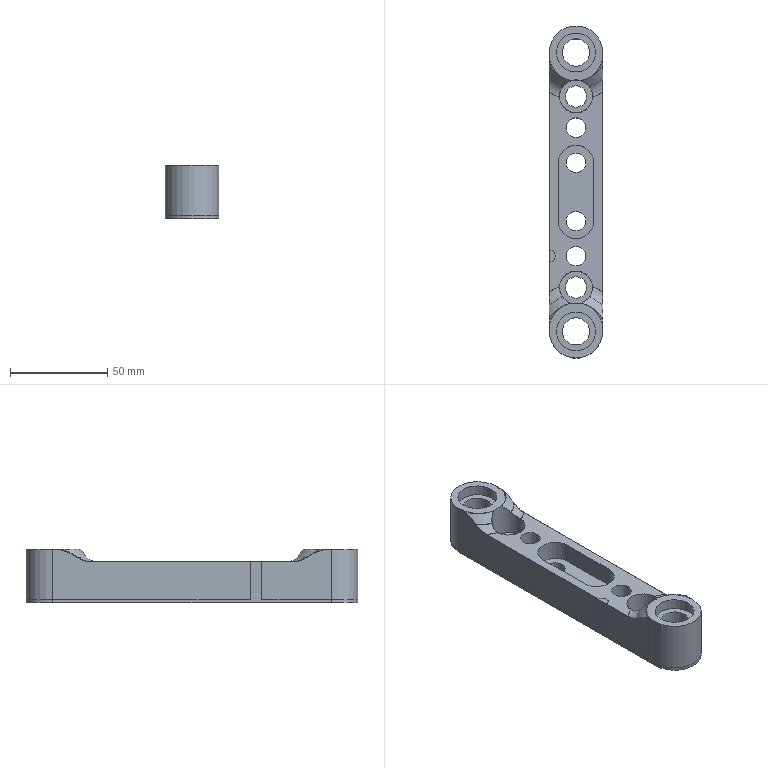NC program | NX | posted with a generic post | part box 27.4 x 170.48 x 27.5 mm
Whole program:
N10 G17 G21 G94 G90
(ADAPTIVE_MILLING_1 , TOOL : D12开粗)
N12 T05 M6
N14 G54
N16 G17 G0 G90 X0.829 Y-27.07 B0. C0. S4000 M3
N18 G43 Z30. H5
N20 Z3.15
N22 G94 G1 X0.826 Y-26.92 Z2.213 F1500.
N24 X0.824 Y-26.77 Z1.842
N26 X0.821 Y-26.621 Z1.57
N28 X0.819 Y-26.471 Z1.35
N30 X0.816 Y-26.321 Z1.166
N32 X0.814 Y-26.171 Z1.008
N34 X0.811 Y-26.021 Z0.87
N36 X0.809 Y-25.871 Z0.75
N38 X0.806 Y-25.721 Z0.645
N40 X0.803 Y-25.571 Z0.552
N42 X0.801 Y-25.421 Z0.471
N44 X0.798 Y-25.271 Z0.4
N46 X0.796 Y-25.121 Z0.34
N48 X0.793 Y-24.971 Z0.288
N50 X0.791 Y-24.821 Z0.245
N52 X0.788 Y-24.671 Z0.211
N54 X0.786 Y-24.521 Z0.184
N56 X0.783 Y-24.371 Z0.165
N58 X0.781 Y-24.221 Z0.154
N60 X0.778 Y-24.071 Z0.15
N62 X0.746 Y-22.161
N64 G3 X-0.031 Y-21.05 R1.212
N66 X-2.33 Y-20.671 R8.892
N68 X-10.092 Y-20.505 R127.75
N70 G1 X-15.893 Y-20.5
N72 X-87.518 Y-20.498
N74 G2 X-92.761 Y-17.88 R6.758
N76 X-94.899 Y-13.073 R11.037
N78 X-95.437 Y-7.231 R33.694
N80 X-95.5 Y3.519 R602.199
N82 G1 X-95.485 Y12.901
N84 G2 X-92.826 Y17.806 R6.795
N86 X-88.066 Y19.901 R11.093
N88 X-82.223 Y20.437 R33.794
N90 X-71.536 Y20.5 R606.615
N92 G1 X87.513 Y20.498
N94 G2 X92.718 Y17.932 R6.744
N96 X94.898 Y13.077 R10.99
N98 X95.437 Y7.234 R33.651
N100 X95.5 Y-3.515 R599.847
N102 X95.477 Y-13.012 R452.183
N104 X92.737 Y-17.875 R6.838
N106 X87.893 Y-19.935 R11.296
N108 X81.922 Y-20.445 R36.063
N110 X71.485 Y-20.5 R687.258
N112 G1 X2.685 Y-20.498
N114 G2 X-2.555 Y-20.179 R207.713
N116 G3 X-13.709 Y-20.002 R241.301
N118 G1 X-85.206 Y-20.
N120 G2 X-92.335 Y-16.169 R8.493
N122 X-94.399 Y-10.848 R13.645
N124 X-94.943 Y-4.127 R42.959
N126 X-94.981 Y10.828 R775.097
N128 X-91.119 Y17.37 R8.52
N130 X-85.665 Y19.432 R13.856
N132 X-79.129 Y19.943 R44.253
N134 X-67.941 Y19.999 R711.37
N136 G1 X85.391 Y19.998
N138 G2 X92.32 Y16.193 R8.497
N140 X94.419 Y10.74 R13.731
N142 X94.945 Y4.018 R44.185
N144 X94.981 Y-10.829 R775.196
N146 X91.193 Y-17.32 R8.514
N148 X85.74 Y-19.419 R13.731
N150 X79.018 Y-19.945 R44.185
N152 X68.018 Y-19.999 R708.841
N154 G1 X4.546 Y-19.998
N156 G2 X-2.571 Y-19.689 R193.168
N158 G3 X-17.331 Y-19.501 R359.212
N160 G1 X-83.318 Y-19.499
N162 G2 X-92.049 Y-14.514 R9.751
N164 X-93.974 Y-8.669 R16.306
N166 X-94.452 Y-1.44 R55.525
N168 X-94.475 Y9.059 R350.5
N170 X-89.782 Y16.886 R9.65
N172 X-84.163 Y18.893 R15.539
N174 X-77.003 Y19.442 R48.976
N176 X-65.878 Y19.499 R709.869
N178 G1 X83.297 Y19.498
N180 G2 X92.044 Y14.522 R9.746
N182 X93.973 Y8.675 R16.302
N184 X94.454 Y1.321 R56.162
N186 X94.475 Y-9.053 R349.283
N188 X89.62 Y-16.985 R9.68
N190 X83.917 Y-18.935 R15.94
N192 X76.504 Y-19.451 R53.271
N194 X66.816 Y-19.499 R682.89
N196 G1 X6.296 Y-19.498
N198 G2 X-2.421 Y-19.201 R210.628
N200 G3 X-17.581 Y-19.001 R393.774
N202 G1 X-81.393 Y-19.
N204 G2 X-86.346 Y-18.142 R12.42
N206 X-91.86 Y-12.747 R10.926
N208 X-93.556 Y-6.563 R19.418
N210 X-93.969 Y1.61 R74.972
N212 X-93.95 Y7.796 R113.708
N214 X-88.474 Y16.474 R10.528
N216 X-82.381 Y18.442 R17.533
N218 X-74.591 Y18.952 R59.673
N220 X-63.591 Y18.999 R733.727
N222 G1 X81.454 Y18.997
N224 G2 X86.517 Y18.067 R12.222
N226 X91.865 Y12.735 R10.951
N228 X93.55 Y6.613 R19.369
N230 X93.968 Y-1.56 R74.178
N232 X93.949 Y-7.809 R112.262
N234 X88.46 Y-16.481 R10.53
N236 X82.541 Y-18.417 R17.383
N238 X75.003 Y-18.944 R56.215
N240 X63.628 Y-18.999 R730.673
N242 G1 X7.421 Y-18.997
N244 G2 X-2.831 Y-18.691 R281.614
N246 G3 X-17.644 Y-18.501 R447.13
N248 G1 X-79.456
N250 G2 X-84.043 Y-18.034 R17.16
N252 X-90.983 Y-12.394 R11.224
N254 X-92.935 Y-6.098 R18.884
N256 X-93.449 Y1.88 R63.283
N258 X-93.396 Y6.94 R52.399
N260 X-87.397 Y15.979 R11.191
N262 X-81.102 Y17.934 R18.844
N264 X-73.186 Y18.448 R62.931
N266 X-62.186 Y18.498 R726.714
N268 G1 X79.829 Y18.497
N270 G2 X84.639 Y17.853 R15.103
N272 X91.07 Y12.229 R11.305
N274 X92.953 Y5.968 R19.244
N276 X93.452 Y-2.073 R65.544
N278 X93.396 Y-6.946 R49.972
N280 X87.397 Y-15.979 R11.191
N282 X81.035 Y-17.943 R18.96
N284 X73.182 Y-18.448 R63.488
N286 X61.807 Y-18.498 R740.564
N288 G1 X8.796
N290 G2 X-3.309 Y-18.179 R348.204
N292 G3 X-19.643 Y-18.002 R537.591
N294 G1 X-78.255 Y-18.
N296 G2 X-83.15 Y-17.476 R18.424
N298 X-90.439 Y-11.481 R11.762
N300 X-92.407 Y-5.059 R19.787
N302 X-92.895 Y5.417 R63.029
N304 X-89.815 Y12.904 R11.805
N306 X-83.663 Y16.603 R13.98
N308 X-76.774 Y17.753 R30.115
N310 X-65.591 Y17.993 R181.42
N312 G1 X-60.091 Y17.998
N314 X78.079 Y17.997
N316 G2 X82.858 Y17.549 R19.625
N318 X90.38 Y11.591 R11.715
N320 X92.398 Y5.116 R19.602
N322 X92.895 Y-5.422 R62.792
N324 X89.814 Y-12.904 R11.817
N326 X83.658 Y-16.603 R13.98
N328 X76.707 Y-17.757 R30.295
N330 X66.086 Y-17.992 R175.506
N332 G1 X59.898 Y-17.998
N334 X9.848 Y-17.997
N336 G2 X-3.239 Y-17.685 R373.536
N338 G3 X-20.705 Y-17.502 R591.226
N340 G1 X-76.568 Y-17.501
N342 G2 X-81.482 Y-17.124 R23.942
N344 X-89.789 Y-10.826 R12.167
N346 X-91.869 Y-4.178 R20.227
N348 X-92.337 Y4.484 R46.284
N350 X-89.35 Y12.009 R12.28
N352 X-83.184 Y15.926 R14.111
N354 X-76.255 Y17.199 R29.02
N356 X-66.074 Y17.487 R144.177
N358 G1 X-58.512 Y17.497
N360 X76.579
N362 G2 X81.554 Y17.106 R23.62
N364 X89.828 Y10.751 R12.177
N366 X91.855 Y4.257 R20.245
N368 X92.329 Y-4.591 R45.343
N370 X88.885 Y-12.504 R12.178
N372 X82.709 Y-16.077 R14.638
N374 X75.82 Y-17.232 R31.06
N376 X65.45 Y-17.489 R162.531
N378 G1 X59.263 Y-17.497
N380 X10.963
N382 G2 X-3.294 Y-17.187 R421.689
N384 G3 X-21.705 Y-17.002 R648.175
N386 G1 X-75.193 Y-17.001
N388 G2 X-80.36 Y-16.644 R27.543
N390 X-89.302 Y-9.911 R12.611
N392 X-91.348 Y-3.241 R21.064
N394 X-91.737 Y3.86 R33.584
N396 X-85.009 Y14.237 R12.456
N398 X-78.475 Y16.31 R20.55
N400 X-70.191 Y16.923 R62.181
N402 X-57.442 Y16.997 R743.168
N404 G1 X75.204 Y16.996
N406 G2 X80.371 Y16.639 R27.444
N408 X89.301 Y9.912 R12.608
N410 X91.366 Y3.118 R21.214
N412 X91.736 Y-3.859 R33.428
N414 X84.929 Y-14.279 R12.472
N416 X78.197 Y-16.352 R20.968
N418 X69.598 Y-16.936 R67.204
N420 X57.223 Y-16.997 R755.549
N422 G1 X11.236 Y-16.996
N424 G2 X-4.276 Y-16.664 R552.249
N426 G3 X-21.768 Y-16.502 R716.955
N428 G1 X-73.193
N430 G2 X-78.559 Y-16.275 R41.224
N432 X-88.84 Y-8.98 R13.072
N434 X-90.88 Y-1.992 R22.207
N436 X-91.005 Y4.175 R22.482
N438 X-84.59 Y13.488 R12.567
N440 X-77.801 Y15.753 R20.426
N442 X-69.333 Y16.415 R60.92
N444 X-55.834 Y16.497 R701.757
N446 G1 X74.017 Y16.496
N448 G2 X79.311 Y16.154 R30.394
N450 X88.748 Y9.156 R12.989
N452 X90.843 Y2.242 R21.743
N454 X91.022 Y-4.048 R23.09
N456 X84.439 Y-13.572 R12.6
N458 X77.697 Y-15.769 R20.722
N460 X69.478 Y-16.411 R61.005
N462 X55.979 Y-16.497 R664.152
N464 G1 X12.116 Y-16.495
N466 G2 X-4.519 Y-16.161 R601.24
N468 G3 X-22.955 Y-16.002 R784.695
N470 G1 X-72.443 Y-16.001
N472 G2 X-77.931 Y-15.727 R38.534
N474 X-88.225 Y-8.377 R13.376
N476 X-90.425 Y2.899 R21.949
N478 X-83.927 Y12.886 R12.7
N480 X-77.033 Y15.218 R20.695
N482 X-68.568 Y15.905 R60.492
N484 X-54.818 Y15.996 R638.782
N486 G1 X72.857 Y15.995
N488 G2 X78.34 Y15.658 R33.247
N490 X88.223 Y8.378 R13.347
N492 X90.456 Y-0.151 R22.185
N494 X89.289 Y-7.165 R14.254
N496 X83.094 Y-13.333 R13.169
N498 X76.154 Y-15.355 R22.709
N500 X67.366 Y-15.932 R72.607
N502 X54.741 Y-15.996 R761.795
N504 G1 X12.941 Y-15.995
N506 G2 X-4.472 Y-15.664 R634.391
N508 G3 X-23.643 Y-15.502 R830.844
N510 G1 X-71.13 Y-15.501
N512 G2 X-76.87 Y-15.245 R44.05
N514 X-84.754 Y-11.622 R13.869
N516 X-88.857 Y-4.771 R15.871
N518 X-89.672 Y2.816 R18.197
N520 X-83.509 Y12.146 R12.666
N522 X-76.655 Y14.617 R20.217
N524 X-68.323 Y15.38 R55.67
N526 X-53.699 Y15.496 R534.547
N528 G1 X71.579 Y15.495
N530 G2 X77.314 Y15.176 R37.451
N532 X87.719 Y7.585 R13.689
N534 X89.728 Y-2.283 R19.122
N536 X83.515 Y-12.14 R12.664
N538 X76.668 Y-14.613 R20.182
N540 X68.523 Y-15.373 R54.802
N542 X53.399 Y-15.496 R522.551
N544 G1 X13.787 Y-15.495
N546 G2 X-3.396 Y-15.192 R584.055
N548 G3 X-24.455 Y-15.002 R846.592
N550 G1 X-69.818
N552 G2 X-75.809 Y-14.765 R50.716
N554 X-83.264 Y-11.792 R14.564
N556 X-88.121 Y-4.615 R15.31
N558 X-88.809 Y3.084 R15.479
N560 X-83.006 Y11.451 R12.602
N562 X-76.258 Y14.017 R19.783
N564 X-67.997 Y14.855 R52.035
N566 X-52.498 Y14.996 R477.394
N568 G1 X70.391 Y14.995
N570 G2 X76.316 Y14.691 R41.594
N572 X84.657 Y10.51 R14.034
N574 X88.76 Y2.15 R16.573
N576 X87.99 Y-5.758 R13.481
N578 X82.063 Y-12.003 R13.135
N580 X75.183 Y-14.213 R21.962
N582 X66.467 Y-14.903 R64.14
N584 X52.343 Y-14.996 R664.847
N586 G1 X14.605 Y-14.995
N588 G2 X-4.696 Y-14.664 R707.553
N590 G3 X-25.205 Y-14.502 R877.026
N592 G1 X-68.63
N594 G2 X-74.997 Y-14.256 R54.441
N596 X-82.285 Y-11.494 R15.033
N598 X-88.191 Y1.216 R15.106
N600 X-82.844 Y10.515 R12.292
N602 X-76.152 Y13.349 R18.763
N604 X-68.032 Y14.311 R46.434
N606 X-53.972 Y14.494 R340.479
N608 G1 X68.641 Y14.495
N610 G2 X74.822 Y14.272 R56.066
N612 X81.882 Y11.779 R15.278
N614 X87.673 Y3.458 R14.94
N616 X87.345 Y-4.943 R12.977
N618 X81.596 Y-11.306 R12.961
N620 X74.697 Y-13.641 R21.444
N622 X66.112 Y-14.384 R60.341
N624 X50.863 Y-14.495 R595.661
N626 G1 X15.25 Y-14.494
N628 G2 X-3.451 Y-14.193 R667.873
N630 G3 X-24.331 Y-14.003 R861.877
N632 G1 X-67.443 Y-14.002
N634 G2 X-73.998 Y-13.772 R60.539
N636 X-81.03 Y-11.374 R15.782
N638 X-87.357 Y0.017 R14.091
N640 X-82.546 Y9.633 R11.937
N642 X-76.002 Y12.674 R17.87
N644 X-68.088 Y13.758 R41.645
N646 X-55.342 Y13.991 R248.601
N648 G1 X-49.842 Y13.995
N650 X68.204 Y13.994
N652 G2 X74.505 Y13.703 R48.626
N654 X82.052 Y10.629 R15.072
N656 X87.354 Y-0.079 R14.064
N658 X82.546 Y-9.63 R11.936
N660 X75.881 Y-12.702 R17.974
N662 X67.963 Y-13.764 R42.466
N664 X55.217 Y-13.991 R255.149
N666 G1 X49.717 Y-13.995
N668 X15.292 Y-13.993
N670 G2 X-4.564 Y-13.669 R790.323
N672 G3 X-25.455 Y-13.503 R889.408
N674 G1 X-66.818 Y-13.501
N676 G2 X-73.434 Y-13.239 R56.881
N678 X-80.607 Y-10.686 R15.86
N680 X-86.367 Y-1.378 R13.262
N682 X-82.308 Y8.645 R11.482
N684 X-75.782 Y12. R16.935
N686 X-67.951 Y13.208 R38.175
N688 X-55.457 Y13.488 R208.166
N690 G1 X-48.582 Y13.495
N692 X67.079 Y13.494
N694 G2 X73.507 Y13.225 R54.065
N696 X80.774 Y10.567 R15.737
N698 X86.367 Y1.357 R13.238
N700 X82.324 Y-8.627 R11.468
N702 X75.856 Y-11.976 R16.879
N704 X68.216 Y-13.189 R37.305
N706 X56.035 Y-13.486 R192.639
N708 G1 X49.847 Y-13.494
N710 X15.985 Y-13.493
N712 G2 X-4.625 Y-13.17 R813.236
N714 G3 X-25.518 Y-13.003 R891.847
N716 G1 X-65.005 Y-13.002
N718 G2 X-72.062 Y-12.799 R76.266
N720 X-78.862 Y-10.832 R17.251
N722 X-85.044 Y-3.276 R12.786
N724 X-82.194 Y7.439 R10.91
N726 X-76.092 Y11.131 R15.503
N728 X-68.624 Y12.583 R31.93
N730 X-58.072 Y12.969 R133.493
N732 G1 X-47.759 Y12.994
N734 X65.954 Y12.993
N736 G2 X72.571 Y12.739 R59.378
N738 X79.621 Y10.374 R16.369
N740 X85.183 Y2.72 R12.564
N742 X82.139 Y-7.492 R10.93
N744 X75.949 Y-11.177 R15.622
N746 X68.475 Y-12.595 R32.584
N748 X57.796 Y-12.972 R138.128
N750 G1 X47.484 Y-12.994
N752 X16.621 Y-12.993
N754 G2 X-4.871 Y-12.666 R884.109
N756 G3 X-25.581 Y-12.503 R894.734
N758 G1 X-64.118 Y-12.502
N760 G2 X-71.362 Y-12.288 R77.142
N762 X-78.052 Y-10.391 R17.565
N764 X-83.724 Y-4.176 R12.144
N766 X-81.731 Y6.455 R10.376
N768 X-75.696 Y10.457 R14.697
N770 X-68.504 Y12.005 R29.512
N772 X-58.205 Y12.459 R113.868
N774 G1 X-47.893 Y12.494
N776 X64.907 Y12.493
N778 G2 X71.65 Y12.252 R64.503
N780 X78.528 Y10.118 R16.965
N782 X83.868 Y3.77 R11.941
N784 X81.685 Y-6.503 R10.394
N786 X75.715 Y-10.446 R14.704
N788 X68.524 Y-12.001 R29.475
N790 X58.037 Y-12.46 R114.611
N792 G1 X47.725 Y-12.494
N794 X17.175 Y-12.493
N796 G2 X-4.932 Y-12.166 R931.379
N798 G3 X-25.831 Y-12.003 R904.563
N800 G1 X-63.618 Y-12.002
N802 G2 X-70.798 Y-11.764 R71.881
N804 X-77.48 Y-9.818 R17.487
N806 X-82.557 Y-4.359 R11.272
N808 X-81.167 Y5.455 R9.846
N810 X-75.423 Y9.705 R13.739
N812 X-68.524 Y11.398 R26.554
N814 X-58.793 Y11.938 R92.598
N816 X-45.543 Y11.994 R809.607
N818 G1 X63.819 Y11.993
N820 G2 X70.936 Y11.743 R67.913
N822 X77.596 Y9.75 R17.236
N824 X82.647 Y4.125 R11.179
N826 X81.087 Y-5.553 R9.87
N828 X75.424 Y-9.7 R13.791
N830 X68.464 Y-11.403 R26.649
N832 X59.17 Y-11.931 R90.613
N834 X46.608 Y-11.993 R770.861
N836 G1 X17.746 Y-11.992
N838 G2 X-4.805 Y-11.67 R932.733
N840 G3 X-25.331 Y-11.504 R897.593
N842 G1 X-61.931 Y-11.503
N844 G2 X-69.551 Y-11.309 R92.814
N846 X-75.894 Y-9.76 R18.889
N848 X-80.962 Y-5.227 R10.914
N850 X-80.366 Y4.616 R9.332
N852 X-74.933 Y9.001 R12.937
N854 X-68.071 Y10.835 R24.655
N856 X-58.907 Y11.418 R81.712
N858 X-45.657 Y11.493 R768.448
N860 G1 X62.893
N862 G2 X70.073 Y11.252 R72.048
N864 X76.477 Y9.468 R17.672
N866 X81.298 Y4.542 R10.49
N868 X80.285 Y-4.725 R9.373
N870 X74.862 Y-9.028 R13.027
N872 X68.18 Y-10.818 R24.611
N874 X58.955 Y-11.417 R80.295
N876 X45.643 Y-11.493 R767.874
N878 G1 X18.156 Y-11.492
N880 G2 X-4.866 Y-11.169 R947.356
N882 G3 X-25.393 Y-11.004 R902.187
N884 G1 X-60.993 Y-11.003
N886 G2 X-68.801 Y-10.807 R95.868
N888 X-74.975 Y-9.346 R18.958
N890 X-79.749 Y-5.112 R9.996
N892 X-79.352 Y3.932 R8.886
N894 X-74.212 Y8.362 R12.285
N896 X-67.503 Y10.28 R23.032
N898 X-58.593 Y10.904 R74.373
N900 X-44.843 Y10.993 R734.904
N902 G1 X61.957 Y10.992
N904 G2 X69.387 Y10.743 R74.063
N906 X75.394 Y9.142 R17.639
N908 X80.099 Y4.381 R9.655
N910 X79.174 Y-4.196 R8.967
N912 X73.907 Y-8.501 R12.526
N914 X67.112 Y-10.334 R24.092
N916 X57.886 Y-10.919 R81.579
N918 X44.574 Y-10.993 R772.827
N920 G1 X18.649 Y-10.991
N922 G2 X-5.3 Y-10.662 R994.052
N924 G3 X-25.831 Y-10.504 R912.433
N926 G1 X-59.993 Y-10.503
N928 G2 X-68.051 Y-10.306 R100.864
N930 X-73.821 Y-9.016 R18.909
N932 X-78.478 Y-4.912 R9.163
N934 X-78.107 Y3.449 R8.502
N936 X-73.046 Y7.897 R11.84
N938 X-66.461 Y9.786 R22.439
N940 X-57.301 Y10.411 R75.525
N942 X-43.926 Y10.492 R760.679
N944 G1 X61.061
N946 G2 X68.554 Y10.251 R77.849
N948 X74.226 Y8.829 R17.51
N950 X78.93 Y3.857 R8.814
N952 X77.815 Y-3.893 R8.656
N954 X72.616 Y-8.094 R12.255
N956 X66.118 Y-9.833 R23.65
N958 X56.704 Y-10.423 R81.722
N960 X44.08 Y-10.492 R758.046
N962 G1 X19.155 Y-10.491
N964 G2 X-4.988 Y-10.169 R984.717
N966 G3 X-25.518 Y-10.005 R909.189
N968 G1 X-59.056 Y-10.003
N970 G2 X-67.177 Y-9.816 R107.934
N972 X-72.543 Y-8.707 R18.797
N974 X-77.239 Y-4.365 R8.321
N976 X-76.514 Y3.344 R8.224
N978 X-71.462 Y7.589 R11.681
N980 X-64.972 Y9.349 R22.769
N982 X-56.057 Y9.916 R79.054
N984 X-42.745 Y9.992 R769.559
N986 G1 X60.118 Y9.991
N988 G2 X67.674 Y9.764 R83.297
N990 X72.889 Y8.556 R17.17
N992 X77.606 Y3.294 R8.076
N994 X76.146 Y-3.87 R8.434
N996 X70.956 Y-7.808 R12.195
N998 X64.484 Y-9.411 R24.423
N1000 X55.065 Y-9.934 R89.83
N1002 X41.816 Y-9.992 R805.162
N1004 G1 X19.641 Y-9.991
N1006 G2 X-4.179 Y-9.685 R957.817
N1008 G3 X-26.768 Y-9.505 R941.904
N1010 G1 X-58.118 Y-9.503
N1012 G2 X-66.364 Y-9.321 R113.471
N1014 X-71.137 Y-8.405 R18.024
N1016 X-76.028 Y-3.044 R7.526
N1018 X-74.428 Y3.728 R8.198
N1020 X-69.263 Y7.486 R12.01
N1022 X-62.64 Y8.999 R25.188
N1024 X-52.967 Y9.45 R103.595
N1026 X-41.905 Y9.491 R763.579
N1028 G1 X59.833 Y9.49
N1030 G2 X67.138 Y9.242 R76.193
N1032 X71.74 Y8.15 R15.007
N1034 X75.73 Y-1.322 R7.447
N1036 X71.585 Y-6.294 R9.974
N1038 X65.647 Y-8.537 R17.371
N1040 X57.634 Y-9.341 R50.971
N1042 X42.073 Y-9.492 R472.746
N1044 G1 X20.148 Y-9.491
N1046 G2 X-3.992 Y-9.189 R962.566
N1048 G3 X-26.581 Y-9.005 R942.884
N1050 G1 X-57.243 Y-9.003
N1052 G2 X-65.552 Y-8.825 R117.859
N1054 X-69.659 Y-8.076 R15.977
N1056 X-74.089 Y0.533 R7.011
N1058 X-70.248 Y5.687 R9.332
N1060 X-64.427 Y8.023 R16.092
N1062 X-56.979 Y8.823 R46.053
N1064 X-43.48 Y8.99 R363.158
N1066 G1 X57.57 Y8.991
N1068 G2 X65.628 Y8.811 R110.542
N1070 X69.789 Y8.019 R15.321
N1072 X74.099 Y-0.447 R6.996
N1074 X70.328 Y-5.622 R9.269
N1076 X64.581 Y-7.986 R15.813
N1078 X56.949 Y-8.824 R45.381
N1080 X43.638 Y-8.99 R358.778
N1082 G1 X22.651 Y-8.991
N1084 G2 X-3.057 Y-8.707 R949.688
N1086 G3 X-27.705 Y-8.505 R976.383
N1088 G1 X-56.368 Y-8.503
N1090 G2 X-64.801 Y-8.324 R118.609
N1092 X-68.222 Y-7.649 R11.571
N1094 X-72.154 Y-0.275 R6.558
N1096 X-68.743 Y5.014 R8.672
N1098 X-63.345 Y7.428 R14.389
N1100 X-56.284 Y8.298 R38.91
N1102 X-42.474 Y8.489 R316.862
N1104 G1 X56.701 Y8.491
N1106 G2 X64.822 Y8.314 R112.705
N1108 X68.298 Y7.608 R11.238
N1110 X72.154 Y0.359 R6.549
N1112 X68.821 Y-4.945 R8.637
N1114 X63.276 Y-7.441 R14.348
N1116 X56.087 Y-8.307 R39.838
N1118 X42.464 Y-8.49 R327.538
N1120 G1 X22.977 Y-8.491
N1122 G2 X-2.059 Y-8.226 R936.273
N1124 G3 X-26.706 Y-8.006 R965.075
N1126 G1 X-55.556 Y-8.004
N1128 G2 X-63.74 Y-7.843 R123.986
N1130 X-67.575 Y-6.513 R6.71
N1132 X-69.72 Y-0.225 R6.289
N1134 X-66.279 Y4.828 R8.463
N1136 X-60.777 Y7.111 R14.395
N1138 X-53.636 Y7.851 R42.972
N1140 X-38.075 Y7.99 R480.797
N1142 G1 X57.225 Y7.989
N1144 G2 X64.219 Y7.79 R80.874
N1146 X69.837 Y1.211 R6.078
N1148 X67.029 Y-4.214 R7.996
N1150 X61.768 Y-6.869 R12.808
N1152 X55.217 Y-7.776 R33.214
N1154 X42.97 Y-7.987 R244.19
N1156 G1 X38.158 Y-7.991
N1158 X20.67 Y-7.989
N1160 G2 X-2.507 Y-7.718 R949.008
N1162 G3 X-27.143 Y-7.506 R975.899
N1164 G1 X-54.556 Y-7.504
N1166 G2 X-62.116 Y-7.384 R130.423
N1168 X-66.961 Y-2.502 R5.479
N1170 X-65.04 Y3.182 R7.22
N1172 X-60.131 Y6.199 R11.047
N1174 X-54.171 Y7.226 R25.759
N1176 X-43.988 Y7.48 R157.535
N1178 G1 X-36.613 Y7.49
N1180 X56.374 Y7.489
N1182 G2 X62.122 Y7.372 R96.14
N1184 X66.936 Y2.46 R5.475
N1186 X64.942 Y-3.26 R7.243
N1188 X60.067 Y-6.212 R11.101
N1190 X54.042 Y-7.233 R26.091
N1192 X43.172 Y-7.483 R172.764
N1194 G1 X36.422 Y-7.49
N1196 X20.997 Y-7.488
N1198 G2 X-2.493 Y-7.218 R961.85
N1200 G3 X-26.207 Y-7.006 R961.26
N1202 G1 X-48.193
N1204 G2 X-59.055 Y-6.962 R570.574
N1206 X-63.178 Y-3.457 R4.799
N1208 X-62.166 Y2.133 R6.537
N1210 X-57.558 Y5.558 R9.683
N1212 X-51.878 Y6.708 R21.018
N1214 X-42.322 Y6.98 R127.558
N1216 G1 X-34.885 Y6.99
N1218 X55.528 Y6.988
N1220 G2 X59.214 Y6.929 R50.196
N1222 X63.141 Y3.435 R4.808
N1224 X62.112 Y-2.152 R6.544
N1226 X57.47 Y-5.577 R9.71
N1228 X51.912 Y-6.703 R20.985
N1230 X43.419 Y-6.974 R113.103
N1232 G1 X34.794 Y-6.99
N1234 X-33.494 Y-6.986
N1236 G3 X-37.69 Y-6.578 R21.858
N1238 X-53.097 Y-6.504 R748.607
N1240 G2 X-55.281 Y-6.455 R17.851
N1242 X-57.99 Y-4.416 R4.037
N1244 X-57.499 Y2.116 R5.941
N1246 X-52.944 Y5.275 R9.555
N1248 X-47.487 Y6.275 R21.187
N1250 X-38.866 Y6.482 R135.279
N1252 G1 X-32.241 Y6.489
N1254 X54.704 Y6.488
N1256 G2 X57.677 Y4.78 R3.726
N1258 X57.703 Y-1.706 R5.85
N1260 X53.437 Y-5.063 R8.962
N1262 X48.017 Y-6.227 R18.773
N1264 X39.398 Y-6.48 R111.008
N1266 G1 X32.773 Y-6.49
N1268 X-30.839 Y-6.487
N1270 G2 X-36.394 Y-6.159 R433.547
N1272 G3 X-49.209 Y-6.003 R335.527
N1274 G2 X-51.113 Y-4.87 R3.64
N1276 X-52.121 Y1.25 R5.669
N1278 X-48.085 Y5.024 R6.893
N1280 X-42.657 Y5.835 R24.208
N1282 X-32.909 Y5.987 R202.148
N1284 G1 X-28.784 Y5.989
N1286 X49.079 Y5.985
N1288 G2 X50.934 Y4.89 R3.563
N1290 X51.975 Y-1.223 R5.66
N1292 X47.436 Y-5.227 R7.159
N1294 X43.617 Y-5.815 R15.303
N1296 X33.182 Y-5.988 R195.906
N1298 G1 X-28.517 Y-5.989
N1300 G2 X-35.639 Y-5.704 R156.088
N1302 G3 X-36.996 Y-5.776 R8.044
N1304 G2 X-40.431 Y-5.908 R420.211
N1306 G3 X-41.002 Y-6.059 R1.343
N1308 X-41.38 Y-8.096 Z0.25 R1.322
N1310 X-39.107 Y-7.55 R1.32 F15000.
N1312 G1 X-37.927 Y-2.871
N1314 X-37.344 Y-0.561 Z0.15 F1500.
N1316 X-37.249 Y-0.183
N1318 G3 X-36.798 Y1.183 R34.136
N1320 G2 X-32.368 Y5.2 R6.905
N1322 X-25.313 Y5.473 R73.748
N1324 G1 X-16.688 Y5.489
N1326 X33.937 Y5.492
N1328 G2 X37.915 Y5.841 R22.069
N1330 G1 X39.79 Y5.878
N1332 X39.94 Y5.881 Z0.154
N1334 X40.09 Y5.884 Z0.165
N1336 X40.24 Y5.887 Z0.184
N1338 X40.39 Y5.891 Z0.211
N1340 X40.54 Y5.894 Z0.245
N1342 X40.69 Y5.897 Z0.288
N1344 X40.84 Y5.9 Z0.34
N1346 X40.99 Y5.903 Z0.4
N1348 X41.14 Y5.906 Z0.471
N1350 X41.29 Y5.909 Z0.552
N1352 X41.44 Y5.913 Z0.645
N1354 X41.59 Y5.916 Z0.75
N1356 X41.74 Y5.919 Z0.87
N1358 X41.89 Y5.922 Z1.008
N1360 X42.04 Y5.925 Z1.166
N1362 X42.19 Y5.928 Z1.35
N1364 X42.34 Y5.932 Z1.57
N1366 X42.489 Y5.935 Z1.842
N1368 X42.639 Y5.938 Z2.213
N1370 X42.789 Y5.941 Z3.15
N1372 G0 Z30.
N1374 M5
(PLANAR_MILL_10_COPY_1 , TOOL : D8开粗)
N1376 T06 M6
N1378 G54
N1380 G17 G0 G90 X-72.669 Y-2.779 B0. C0. S3500 M3
N1382 G43 Z30. H6
N1384 Z3.
N1386 G94 G3 X-72.669 Y-2.779 Z2.012 I1.129 J2.779 F800.
N1388 X-72.669 Y-2.779 Z1.024 I1.129 J2.779
N1390 X-72.669 Y-2.779 Z0.036 I1.129 J2.779
N1392 X-72.669 Y-2.779 Z-0.951 I1.129 J2.779
N1394 X-72.669 Y-2.779 Z-1.939 I1.129 J2.779
N1396 X-71.54 Y-3. Z-2. R3.
N1398 X-68.54 Y0. R3.
N1400 X-71.54 Y-3. R-3.
N1402 G1 Y1.
N1404 Z1.
N1406 G0 Z30.
N1408 X72.669 Y2.779
N1410 Z3.
N1412 G3 X72.669 Y2.779 Z2.012 I-1.129 J-2.779
N1414 X72.669 Y2.779 Z1.024 I-1.129 J-2.779
N1416 X72.669 Y2.779 Z0.036 I-1.129 J-2.779
N1418 X72.669 Y2.779 Z-0.951 I-1.129 J-2.779
N1420 X72.669 Y2.779 Z-1.939 I-1.129 J-2.779
N1422 X71.54 Y3. Z-2. R3.
N1424 X68.54 Y0. R3.
N1426 X71.54 Y3. R-3.
N1428 G1 Y-1.
N1430 Z1.
N1432 G0 Z30.
(PLANAR_MILL_10 , TOOL : D8开粗)
N1434 X-72.868 Y1.359
N1436 Z3.
N1438 G3 X-72.868 Y1.359 Z2.374 I1.328 J-1.359
N1440 X-72.868 Y1.359 Z1.749 I1.328 J-1.359
N1442 X-72.868 Y1.359 Z1.123 I1.328 J-1.359
N1444 X-72.868 Y1.359 Z0.497 I1.328 J-1.359
N1446 X-72.868 Y1.359 Z-0.128 I1.328 J-1.359
N1448 X-72.868 Y1.359 Z-0.754 I1.328 J-1.359
N1450 X-72.868 Y1.359 Z-1.38 I1.328 J-1.359
N1452 X-72.868 Y1.359 Z-2.005 I1.328 J-1.359
N1454 X-72.868 Y1.359 Z-2.631 I1.328 J-1.359
N1456 X-72.868 Y1.359 Z-3.256 I1.328 J-1.359
N1458 X-72.868 Y1.359 Z-3.882 I1.328 J-1.359
N1460 X-72.868 Y1.359 Z-4.508 I1.328 J-1.359
N1462 X-72.868 Y1.359 Z-5.133 I1.328 J-1.359
N1464 X-72.868 Y1.359 Z-5.759 I1.328 J-1.359
N1466 X-72.868 Y1.359 Z-6.385 I1.328 J-1.359
N1468 X-72.868 Y1.359 Z-7.01 I1.328 J-1.359
N1470 X-72.868 Y1.359 Z-7.636 I1.328 J-1.359
N1472 X-72.868 Y1.359 Z-8.262 I1.328 J-1.359
N1474 X-72.868 Y1.359 Z-8.887 I1.328 J-1.359
N1476 X-72.868 Y1.359 Z-9.513 I1.328 J-1.359
N1478 X-72.868 Y1.359 Z-10.139 I1.328 J-1.359
N1480 X-72.868 Y1.359 Z-10.764 I1.328 J-1.359
N1482 X-71.54 Y-1.9 Z-11. R1.9
N1484 X-69.64 Y0. R1.9
N1486 X-71.54 Y-1.9 R-1.9
N1488 G1 Y0.1
N1490 Z-8.
N1492 G0 Z30.
N1494 X72.868 Y-1.359
N1496 Z3.
N1498 G3 X72.868 Y-1.359 Z2.374 I-1.328 J1.359
N1500 X72.868 Y-1.359 Z1.749 I-1.328 J1.359
N1502 X72.868 Y-1.359 Z1.123 I-1.328 J1.359
N1504 X72.868 Y-1.359 Z0.497 I-1.328 J1.359
N1506 X72.868 Y-1.359 Z-0.128 I-1.328 J1.359
N1508 X72.868 Y-1.359 Z-0.754 I-1.328 J1.359
N1510 X72.868 Y-1.359 Z-1.38 I-1.328 J1.359
N1512 X72.868 Y-1.359 Z-2.005 I-1.328 J1.359
N1514 X72.868 Y-1.359 Z-2.631 I-1.328 J1.359
N1516 X72.868 Y-1.359 Z-3.256 I-1.328 J1.359
N1518 X72.868 Y-1.359 Z-3.882 I-1.328 J1.359
N1520 X72.868 Y-1.359 Z-4.508 I-1.328 J1.359
N1522 X72.868 Y-1.359 Z-5.133 I-1.328 J1.359
N1524 X72.868 Y-1.359 Z-5.759 I-1.328 J1.359
N1526 X72.868 Y-1.359 Z-6.385 I-1.328 J1.359
N1528 X72.868 Y-1.359 Z-7.01 I-1.328 J1.359
N1530 X72.868 Y-1.359 Z-7.636 I-1.328 J1.359
N1532 X72.868 Y-1.359 Z-8.262 I-1.328 J1.359
N1534 X72.868 Y-1.359 Z-8.887 I-1.328 J1.359
N1536 X72.868 Y-1.359 Z-9.513 I-1.328 J1.359
N1538 X72.868 Y-1.359 Z-10.139 I-1.328 J1.359
N1540 X72.868 Y-1.359 Z-10.764 I-1.328 J1.359
N1542 X71.54 Y1.9 Z-11. R1.9
N1544 X69.64 Y0. R1.9
N1546 X71.54 Y1.9 R-1.9
N1548 G1 Y-0.1
N1550 Z-8.
N1552 G0 Z30.
(PLANAR_MILL_10_COPY , TOOL : D8开粗)
N1554 X-72.209 Y-0.602
N1556 Z-9.
N1558 G1 Z-11. F400.
N1560 G41 X-72.54 Y-0.9 D6
N1562 G3 X-71.54 Y-1.9 R1.
N1564 X-69.64 Y0. R1.9
N1566 X-71.54 Y-1.9 R-1.9
N1568 X-70.54 Y-0.9 R1.
N1570 G40
N1572 G1 X-70.575 Y-0.703
N1574 X-72.505
N1576 G41 X-72.54 Y-0.9
N1578 G3 X-71.54 Y-1.9 R1.
N1580 X-69.64 Y0. R1.9
N1582 X-71.54 Y-1.9 R-1.9
N1584 X-70.54 Y-0.9 R1.
N1586 G40
N1588 G1 X-70.871 Y-0.602
N1590 Z-9.
N1592 G0 Z30.
N1594 X72.209 Y0.602
N1596 Z-9.
N1598 G1 Z-11.
N1600 G41 X72.54 Y0.9
N1602 G3 X71.54 Y1.9 R1.
N1604 X69.64 Y0. R1.9
N1606 X71.54 Y1.9 R-1.9
N1608 X70.54 Y0.9 R1.
N1610 G40
N1612 G1 X70.575 Y0.703
N1614 X72.505
N1616 G41 X72.54 Y0.9
N1618 G3 X71.54 Y1.9 R1.
N1620 X69.64 Y0. R1.9
N1622 X71.54 Y1.9 R-1.9
N1624 X70.54 Y0.9 R1.
N1626 G40
N1628 G1 X70.871 Y0.602
N1630 Z-9.
N1632 G0 Z30.
N1634 M5
(PLANAR_MILL_4 , TOOL : D50R0.8)
N1636 T01 M6
N1638 G54
N1640 G17 G0 G90 X112.24 Y-0.3 B0. C0. S2000 M3
N1642 G43 Z30. H1
N1644 Z2.02
N1646 G94 G1 Z0.02 F600.
N1648 X85.24
N1650 X-85.24
N1652 X-112.24
N1654 Z2.02
N1656 G0 Z30.
N1658 M5
(THREAD_MILLING_1 , TOOL : M10螺纹铣刀)
N1660 T22 M6
N1662 G54
N1664 G17 G0 G90 X-15. Y0. B0. C0. S3000 M3
N1666 G43 Z30. H22
N1668 Z-13.046
N1670 G41 G94 G1 X-14.722 Y0.112 F250. D22
N1672 X-14.705 Y0.126 Z-13.03
N1674 X-14.699 Y0.148 Z-13.015
N1676 X-14.708 Y0.169 Z-13.
N1678 G3 X-14.708 Y0.169 Z-11.5 I-0.292 J-0.169
N1680 G1 X-14.721 Y0.186 Z-11.485
N1682 X-14.743 Y0.193 Z-11.47
N1684 X-14.764 Y0.185 Z-11.454
N1686 G40
N1688 X-15. Y0.
N1690 G0 Z-8.546
N1692 G41 G1 X-14.722 Y0.112
N1694 X-14.705 Y0.126 Z-8.53
N1696 X-14.699 Y0.148 Z-8.515
N1698 X-14.708 Y0.169 Z-8.5
N1700 G3 X-14.708 Y0.169 Z-7. I-0.292 J-0.169
N1702 G1 X-14.721 Y0.186 Z-6.985
N1704 X-14.743 Y0.193 Z-6.97
N1706 X-14.764 Y0.185 Z-6.954
N1708 G40
N1710 X-15. Y0.
N1712 G0 Z-4.046
N1714 G41 G1 X-14.722 Y0.112
N1716 X-14.705 Y0.126 Z-4.03
N1718 X-14.699 Y0.148 Z-4.015
N1720 X-14.708 Y0.169 Z-4.
N1722 G3 X-14.708 Y0.169 Z-2.5 I-0.292 J-0.169
N1724 X-14.708 Y0.169 Z-1. I-0.292 J-0.169
N1726 X-15. Y-0.338 Z0. R-0.338
N1728 G1 X-14.978 Y-0.335 Z0.015
N1730 X-14.962 Y-0.319 Z0.03
N1732 X-14.958 Y-0.297 Z0.046
N1734 G40
N1736 X-15. Y0.
N1738 G0 Z-13.181
N1740 G41 G1 X-14.702 Y-0.031
N1742 G3 X-14.545 Y0.263 Z-13. R0.196
N1744 X-14.545 Y0.263 Z-11.5 I-0.455 J-0.262
N1746 X-14.878 Y0.274 Z-11.319 R0.196
N1748 G40
N1750 G1 X-15. Y0.
N1752 G0 Z-8.681
N1754 G41 G1 X-14.702 Y-0.031
N1756 G3 X-14.545 Y0.263 Z-8.5 R0.196
N1758 X-14.545 Y0.263 Z-7. I-0.455 J-0.262
N1760 X-14.878 Y0.274 Z-6.819 R0.196
N1762 G40
N1764 G1 X-15. Y0.
N1766 G0 Z-4.181
N1768 G41 G1 X-14.702 Y-0.031
N1770 G3 X-14.545 Y0.263 Z-4. R0.196
N1772 X-14.545 Y0.263 Z-2.5 I-0.455 J-0.263
N1774 X-14.545 Y0.263 Z-1. I-0.455 J-0.263
N1776 X-15. Y-0.525 Z0. R-0.525
N1778 X-14.824 Y-0.243 Z0.181 R0.196
N1780 G40
N1782 G1 X-15. Y0.
N1784 G0 Z-13.244
N1786 G41 G1 X-14.721 Y-0.111
N1788 G3 X-14.383 Y0.356 Z-13. R0.316
N1790 X-14.383 Y0.356 Z-11.5 I-0.617 J-0.356
N1792 X-14.957 Y0.297 Z-11.256 R0.316
N1794 G40
N1796 G1 X-15. Y0.
N1798 G0 Z-8.744
N1800 G41 G1 X-14.721 Y-0.111
N1802 G3 X-14.383 Y0.356 Z-8.5 R0.316
N1804 X-14.383 Y0.356 Z-7. I-0.617 J-0.356
N1806 X-14.957 Y0.297 Z-6.756 R0.316
N1808 G40
N1810 G1 X-15. Y0.
N1812 G0 Z-4.244
N1814 G41 G1 X-14.721 Y-0.111
N1816 G3 X-14.383 Y0.356 Z-4. R0.316
N1818 X-14.383 Y0.356 Z-2.5 I-0.617 J-0.356
N1820 X-14.383 Y0.356 Z-1. I-0.617 J-0.356
N1822 X-15. Y-0.713 Z0. R-0.713
N1824 X-14.764 Y-0.186 Z0.244 R0.316
N1826 G40
N1828 G1 X-15. Y0.
N1830 G0 Z-13.278
N1832 G41 G1 X-14.744 Y-0.157
N1834 G3 X-14.221 Y0.45 Z-13. R0.425
N1836 X-14.221 Y0.45 Z-11.5 I-0.779 J-0.45
N1838 X-15.008 Y0.3 Z-11.222 R0.425
N1840 G40
N1842 G1 X-15. Y0.
N1844 G0 Z-8.778
N1846 G41 G1 X-14.744 Y-0.157
N1848 G3 X-14.221 Y0.45 Z-8.5 R0.425
N1850 X-14.221 Y0.45 Z-7. I-0.779 J-0.45
N1852 X-15.008 Y0.3 Z-6.722 R0.425
N1854 G40
N1856 G1 X-15. Y0.
N1858 G0 Z-4.278
N1860 G41 G1 X-14.744 Y-0.157
N1862 G3 X-14.221 Y0.45 Z-4. R0.425
N1864 X-14.221 Y0.45 Z-2.5 I-0.779 J-0.45
N1866 X-14.221 Y0.45 Z-1. I-0.779 J-0.45
N1868 X-15. Y-0.9 Z0. R-0.9
N1870 X-14.736 Y-0.143 Z0.278 R0.425
N1872 G40
N1874 G1 X-15. Y0.
N1876 G0 Z-13.278
N1878 G41 G1 X-14.744 Y-0.157
N1880 G3 X-14.221 Y0.45 Z-13. R0.425
N1882 X-14.221 Y0.45 Z-11.5 I-0.779 J-0.45
N1884 X-15.008 Y0.3 Z-11.222 R0.425
N1886 G40
N1888 G1 X-15. Y0.
N1890 G0 Z-8.778
N1892 G41 G1 X-14.744 Y-0.157
N1894 G3 X-14.221 Y0.45 Z-8.5 R0.425
N1896 X-14.221 Y0.45 Z-7. I-0.779 J-0.45
N1898 X-15.008 Y0.3 Z-6.722 R0.425
N1900 G40
N1902 G1 X-15. Y0.
N1904 G0 Z-4.278
N1906 G41 G1 X-14.744 Y-0.157
N1908 G3 X-14.221 Y0.45 Z-4. R0.425
N1910 X-14.221 Y0.45 Z-2.5 I-0.779 J-0.45
N1912 X-14.221 Y0.45 Z-1. I-0.779 J-0.45
N1914 X-15. Y-0.9 Z0. R-0.9
N1916 X-14.736 Y-0.143 Z0.278 R0.425
N1918 G40
N1920 G1 X-15. Y0.
N1922 G0 Z-13.278
N1924 G41 G1 X-14.744 Y-0.157
N1926 G3 X-14.221 Y0.45 Z-13. R0.425
N1928 X-14.221 Y0.45 Z-11.5 I-0.779 J-0.45
N1930 X-15.008 Y0.3 Z-11.222 R0.425
N1932 G40
N1934 G1 X-15. Y0.
N1936 G0 Z-8.778
N1938 G41 G1 X-14.744 Y-0.157
N1940 G3 X-14.221 Y0.45 Z-8.5 R0.425
N1942 X-14.221 Y0.45 Z-7. I-0.779 J-0.45
N1944 X-15.008 Y0.3 Z-6.722 R0.425
N1946 G40
N1948 G1 X-15. Y0.
N1950 G0 Z-4.278
N1952 G41 G1 X-14.744 Y-0.157
N1954 G3 X-14.221 Y0.45 Z-4. R0.425
N1956 X-14.221 Y0.45 Z-2.5 I-0.779 J-0.45
N1958 X-14.221 Y0.45 Z-1. I-0.779 J-0.45
N1960 X-15. Y-0.9 Z0. R-0.9
N1962 X-14.736 Y-0.143 Z0.278 R0.425
N1964 G40
N1966 G1 X-15. Y0.
N1968 G0 Z30.
N1970 X15.
N1972 Z-13.046
N1974 G41 G1 X15.278 Y0.112
N1976 X15.295 Y0.126 Z-13.03
N1978 X15.301 Y0.148 Z-13.015
N1980 X15.292 Y0.169 Z-13.
N1982 G3 X15.292 Y0.169 Z-11.5 I-0.292 J-0.169
N1984 G1 X15.279 Y0.186 Z-11.485
N1986 X15.257 Y0.193 Z-11.47
N1988 X15.236 Y0.185 Z-11.454
N1990 G40
N1992 X15. Y0.
N1994 G0 Z-8.546
N1996 G41 G1 X15.278 Y0.112
N1998 X15.295 Y0.126 Z-8.53
N2000 X15.301 Y0.148 Z-8.515
N2002 X15.292 Y0.169 Z-8.5
N2004 G3 X15.292 Y0.169 Z-7. I-0.292 J-0.169
N2006 G1 X15.279 Y0.186 Z-6.985
N2008 X15.257 Y0.193 Z-6.97
N2010 X15.236 Y0.185 Z-6.954
N2012 G40
N2014 X15. Y0.
N2016 G0 Z-4.046
N2018 G41 G1 X15.278 Y0.112
N2020 X15.295 Y0.126 Z-4.03
N2022 X15.301 Y0.148 Z-4.015
N2024 X15.292 Y0.169 Z-4.
N2026 G3 X15.292 Y0.169 Z-2.5 I-0.292 J-0.169
N2028 X15.292 Y0.169 Z-1. I-0.292 J-0.169
N2030 X15. Y-0.338 Z0. R-0.338
N2032 G1 X15.022 Y-0.335 Z0.015
N2034 X15.038 Y-0.319 Z0.03
N2036 X15.042 Y-0.297 Z0.046
N2038 G40
N2040 X15. Y0.
N2042 G0 Z-13.181
N2044 G41 G1 X15.298 Y-0.031
N2046 G3 X15.455 Y0.263 Z-13. R0.196
N2048 X15.455 Y0.263 Z-11.5 I-0.455 J-0.262
N2050 X15.122 Y0.274 Z-11.319 R0.196
N2052 G40
N2054 G1 X15. Y0.
N2056 G0 Z-8.681
N2058 G41 G1 X15.298 Y-0.031
N2060 G3 X15.455 Y0.263 Z-8.5 R0.196
N2062 X15.455 Y0.263 Z-7. I-0.455 J-0.262
N2064 X15.122 Y0.274 Z-6.819 R0.196
N2066 G40
N2068 G1 X15. Y0.
N2070 G0 Z-4.181
N2072 G41 G1 X15.298 Y-0.031
N2074 G3 X15.455 Y0.263 Z-4. R0.196
N2076 X15.455 Y0.263 Z-2.5 I-0.455 J-0.263
N2078 X15.455 Y0.263 Z-1. I-0.455 J-0.263
N2080 X15. Y-0.525 Z0. R-0.525
N2082 X15.176 Y-0.243 Z0.181 R0.196
N2084 G40
N2086 G1 X15. Y0.
N2088 G0 Z-13.244
N2090 G41 G1 X15.279 Y-0.111
N2092 G3 X15.617 Y0.356 Z-13. R0.316
N2094 X15.617 Y0.356 Z-11.5 I-0.617 J-0.356
N2096 X15.043 Y0.297 Z-11.256 R0.316
N2098 G40
N2100 G1 X15. Y0.
N2102 G0 Z-8.744
N2104 G41 G1 X15.279 Y-0.111
N2106 G3 X15.617 Y0.356 Z-8.5 R0.316
N2108 X15.617 Y0.356 Z-7. I-0.617 J-0.356
N2110 X15.043 Y0.297 Z-6.756 R0.316
N2112 G40
N2114 G1 X15. Y0.
N2116 G0 Z-4.244
N2118 G41 G1 X15.279 Y-0.111
N2120 G3 X15.617 Y0.356 Z-4. R0.316
N2122 X15.617 Y0.356 Z-2.5 I-0.617 J-0.356
N2124 X15.617 Y0.356 Z-1. I-0.617 J-0.356
N2126 X15. Y-0.713 Z0. R-0.713
N2128 X15.236 Y-0.186 Z0.244 R0.316
N2130 G40
N2132 G1 X15. Y0.
N2134 G0 Z-13.278
N2136 G41 G1 X15.256 Y-0.157
N2138 G3 X15.779 Y0.45 Z-13. R0.425
N2140 X15.779 Y0.45 Z-11.5 I-0.779 J-0.45
N2142 X14.992 Y0.3 Z-11.222 R0.425
N2144 G40
N2146 G1 X15. Y0.
N2148 G0 Z-8.778
N2150 G41 G1 X15.256 Y-0.157
N2152 G3 X15.779 Y0.45 Z-8.5 R0.425
N2154 X15.779 Y0.45 Z-7. I-0.779 J-0.45
N2156 X14.992 Y0.3 Z-6.722 R0.425
N2158 G40
N2160 G1 X15. Y0.
N2162 G0 Z-4.278
N2164 G41 G1 X15.256 Y-0.157
N2166 G3 X15.779 Y0.45 Z-4. R0.425
N2168 X15.779 Y0.45 Z-2.5 I-0.779 J-0.45
N2170 X15.779 Y0.45 Z-1. I-0.779 J-0.45
N2172 X15. Y-0.9 Z0. R-0.9
N2174 X15.264 Y-0.143 Z0.278 R0.425
N2176 G40
N2178 G1 X15. Y0.
N2180 G0 Z-13.278
N2182 G41 G1 X15.256 Y-0.157
N2184 G3 X15.779 Y0.45 Z-13. R0.425
N2186 X15.779 Y0.45 Z-11.5 I-0.779 J-0.45
N2188 X14.992 Y0.3 Z-11.222 R0.425
N2190 G40
N2192 G1 X15. Y0.
N2194 G0 Z-8.778
N2196 G41 G1 X15.256 Y-0.157
N2198 G3 X15.779 Y0.45 Z-8.5 R0.425
N2200 X15.779 Y0.45 Z-7. I-0.779 J-0.45
N2202 X14.992 Y0.3 Z-6.722 R0.425
N2204 G40
N2206 G1 X15. Y0.
N2208 G0 Z-4.278
N2210 G41 G1 X15.256 Y-0.157
N2212 G3 X15.779 Y0.45 Z-4. R0.425
N2214 X15.779 Y0.45 Z-2.5 I-0.779 J-0.45
N2216 X15.779 Y0.45 Z-1. I-0.779 J-0.45
N2218 X15. Y-0.9 Z0. R-0.9
N2220 X15.264 Y-0.143 Z0.278 R0.425
N2222 G40
N2224 G1 X15. Y0.
N2226 G0 Z-13.278
N2228 G41 G1 X15.256 Y-0.157
N2230 G3 X15.779 Y0.45 Z-13. R0.425
N2232 X15.779 Y0.45 Z-11.5 I-0.779 J-0.45
N2234 X14.992 Y0.3 Z-11.222 R0.425
N2236 G40
N2238 G1 X15. Y0.
N2240 G0 Z-8.778
N2242 G41 G1 X15.256 Y-0.157
N2244 G3 X15.779 Y0.45 Z-8.5 R0.425
N2246 X15.779 Y0.45 Z-7. I-0.779 J-0.45
N2248 X14.992 Y0.3 Z-6.722 R0.425
N2250 G40
N2252 G1 X15. Y0.
N2254 G0 Z-4.278
N2256 G41 G1 X15.256 Y-0.157
N2258 G3 X15.779 Y0.45 Z-4. R0.425
N2260 X15.779 Y0.45 Z-2.5 I-0.779 J-0.45
N2262 X15.779 Y0.45 Z-1. I-0.779 J-0.45
N2264 X15. Y-0.9 Z0. R-0.9
N2266 X15.264 Y-0.143 Z0.278 R0.425
N2268 G40
N2270 G1 X15. Y0.
N2272 G0 Z30.
N2274 M5
(PLANAR_MILL_5 , TOOL : D6倒角刀)
N2276 T11 M6
N2278 G54
N2280 G17 G0 G90 X73.54 Y-16.4 B0. C0. S3500 M3
N2282 G43 Z30. H11
N2284 Z0.
N2286 G94 G1 Z-2. F800.
N2288 G3 X71.54 Y-14.4 R2.
N2290 G1 X-71.54
N2292 G2 X-85.94 Y0. R14.4
N2294 X-71.54 Y14.4 R14.4
N2296 G1 X71.54
N2298 G2 X85.94 Y0. R14.4
N2300 X71.54 Y-14.4 R14.4
N2302 G3 X69.54 Y-16.4 R2.
N2304 G1 Z0.
N2306 G0 Z30.
(PLANAR_MILL_5_COPY , TOOL : D6倒角刀)
N2308 X73.54 Y-16.2
N2310 Z0.
N2312 G1 Z-2.
N2314 G3 X71.54 Y-14.2 R2.
N2316 G1 X-71.54
N2318 G2 X-85.74 Y0. R14.2
N2320 X-71.54 Y14.2 R14.2
N2322 G1 X71.54
N2324 G2 X85.74 Y0. R14.2
N2326 X71.54 Y-14.2 R14.2
N2328 G3 X69.54 Y-16.2 R2.
N2330 G1 Z0.
N2332 G0 Z30.
(PLANAR_MILL_6 , TOOL : D6倒角刀)
N2334 X-72.54 Y-3.145
N2336 Z0.
N2338 G1 Z-2. F400.
N2340 Y-5.3
N2342 G3 X-71.54 Y-6.3 R1.
N2344 X-65.24 Y0. R6.3
N2346 X-71.54 Y-6.3 R-6.3
N2348 X-70.54 Y-5.3 R1.
N2350 G1 Y-3.145
N2352 Z0.
N2354 G0 Z30.
N2356 X72.54 Y3.145
N2358 Z0.
N2360 G1 Z-2.
N2362 Y5.3
N2364 G3 X71.54 Y6.3 R1.
N2366 X65.24 Y0. R6.3
N2368 X71.54 Y6.3 R-6.3
N2370 X70.54 Y5.3 R1.
N2372 G1 Y3.145
N2374 Z0.
N2376 G0 Z30.
(PLANAR_MILL_6_COPY , TOOL : D6倒角刀)
N2378 X48. Y-3.458
N2380 Z1.
N2382 G1 Z-1. F800.
N2384 Y-3.6
N2386 G3 X49. Y-4.6 R1.
N2388 X53.6 Y0. R4.6
N2390 X49. Y-4.6 R-4.6
N2392 X50. Y-3.6 R1.
N2394 G1 Y-3.458
N2396 Z1.
N2398 G0 Z30.
N2400 X34. Y2.934
N2402 Z1.
N2404 G1 Z-1.
N2406 Y3.1
N2408 G3 X33. Y4.1 R1.
N2410 X28.9 Y0. R4.1
N2412 X33. Y4.1 R-4.1
N2414 X32. Y3.1 R1.
N2416 G1 Y2.934
N2418 Z1.
N2420 G0 Z30.
N2422 X-32.
N2424 Z1.
N2426 G1 Z-1.
N2428 Y3.1
N2430 G3 X-33. Y4.1 R1.
N2432 X-37.1 Y0. R4.1
N2434 X-33. Y4.1 R-4.1
N2436 X-34. Y3.1 R1.
N2438 G1 Y2.934
N2440 Z1.
N2442 G0 Z30.
N2444 X-50. Y-3.458
N2446 Z1.
N2448 G1 Z-1.
N2450 Y-3.6
N2452 G3 X-49. Y-4.6 R1.
N2454 X-44.4 Y0. R4.6
N2456 X-49. Y-4.6 R-4.6
N2458 X-48. Y-3.6 R1.
N2460 G1 Y-3.458
N2462 Z1.
N2464 G0 Z30.
(PLANAR_MILL_6_COPY_COPY , TOOL : D6倒角刀)
N2466 X-14. Y1.96
N2468 Z0.
N2470 G1 Z-2.
N2472 Y2.2
N2474 G3 X-15. Y3.2 R1.
N2476 X-18.2 Y0. R3.2
N2478 X-15. Y3.2 R-3.2
N2480 X-16. Y2.2 R1.
N2482 G1 Y1.96
N2484 Z0.
N2486 G0 Z30.
N2488 X16.
N2490 Z0.
N2492 G1 Z-2.
N2494 Y2.2
N2496 G3 X15. Y3.2 R1.
N2498 X11.8 Y0. R3.2
N2500 X15. Y3.2 R-3.2
N2502 X14. Y2.2 R1.
N2504 G1 Y1.96
N2506 Z0.
N2508 G0 Z30.
N2510 M5
(PLANAR_MILL_4_COPY , TOOL : D50R0.8)
N2512 T01 M6
N2514 G54
N2516 G17 G0 G90 X112.24 Y-0.3 B0. C0. S2000 M3
N2518 G43 Z30. H1
N2520 Z2.
N2522 G94 G1 Z0. F600.
N2524 X85.24
N2526 X-85.24
N2528 X-112.24
N2530 Z2.
N2532 G0 Z30.
N2534 M5
N2536 M2